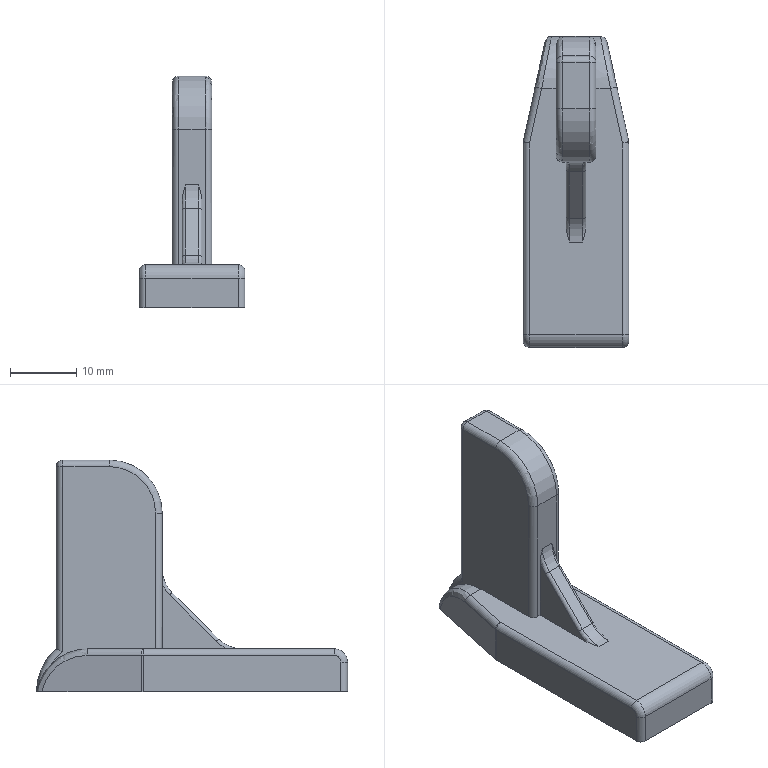Part | STEP file | 101000007607 | 1 solid | 61 faces | box 16 x 47 x 35 mm | volume 7077 mm3 | cylinder 28 | plane 17 | torus 10 | sphere 4 | spline 2 | commonest cylinder face diameters 2 x15 2.5 x4 16 x3 1 x2 10 x2 4 x1